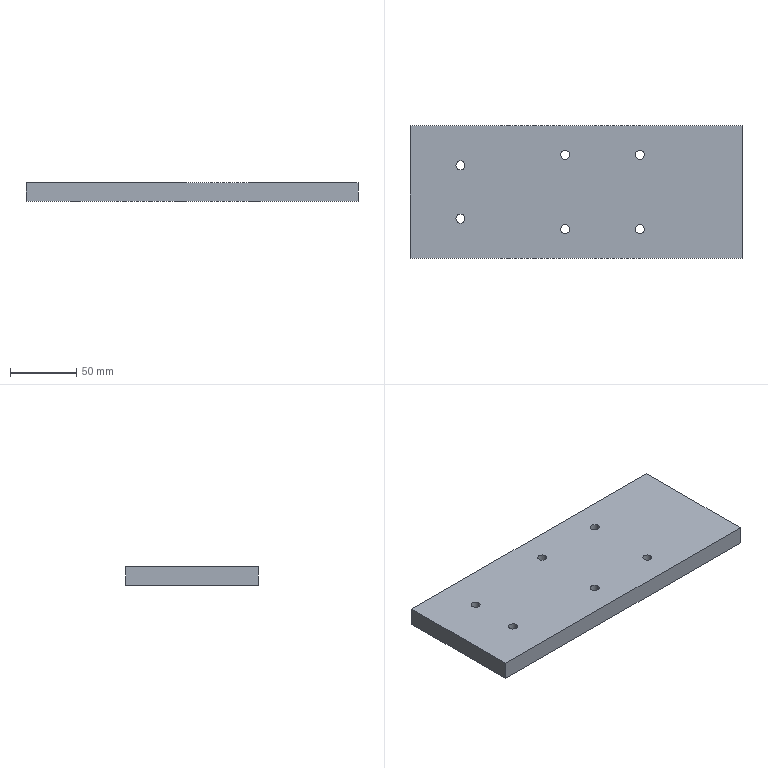Part | SolidWorks | features HoleWzd 2, Extrusion 1 | 1 solid | 18 faces | box 250 x 100 x 14 mm | volume 346949 mm3 | cylinder 12 | plane 6 | commonest cylinder face diameters 6.8 x12
STEP:
#1=CARTESIAN_POINT('',(34.6,70.,0.));
#2=VERTEX_POINT('',#1);
#3=CARTESIAN_POINT('',(41.4,70.,0.));
#4=VERTEX_POINT('',#3);
#5=CARTESIAN_POINT('',(38.,70.,0.));
#6=DIRECTION('',(0.,0.,1.));
#7=DIRECTION('',(1.,0.,0.));
#8=AXIS2_PLACEMENT_3D('',#5,#6,#7);
#9=CIRCLE('',#8,3.4);
#10=EDGE_CURVE('',#2,#4,#9,.T.);
#11=ORIENTED_EDGE('',*,*,#10,.F.);
#12=CARTESIAN_POINT('',(34.6,70.,14.));
#13=VERTEX_POINT('',#12);
#14=CARTESIAN_POINT('',(34.6,70.,14.));
#15=DIRECTION('',(0.,0.,1.));
#16=VECTOR('',#15,1000.);
#17=LINE('',#14,#16);
#18=EDGE_CURVE('',#2,#13,#17,.T.);
#19=ORIENTED_EDGE('',*,*,#18,.T.);
#20=CARTESIAN_POINT('',(41.4,70.,14.));
#21=VERTEX_POINT('',#20);
#22=CARTESIAN_POINT('',(38.,70.,14.));
#23=DIRECTION('',(0.,0.,1.));
#24=DIRECTION('',(1.,0.,0.));
#25=AXIS2_PLACEMENT_3D('',#22,#23,#24);
#26=CIRCLE('',#25,3.4);
#27=EDGE_CURVE('',#13,#21,#26,.T.);
#28=ORIENTED_EDGE('',*,*,#27,.T.);
#29=CARTESIAN_POINT('',(41.4,70.,14.));
#30=DIRECTION('',(0.,0.,1.));
#31=VECTOR('',#30,1000.);
#32=LINE('',#29,#31);
#33=EDGE_CURVE('',#4,#21,#32,.T.);
#34=ORIENTED_EDGE('',*,*,#33,.F.);
#35=EDGE_LOOP('',(#11,#19,#28,#34));
#36=FACE_OUTER_BOUND('',#35,.T.);
#37=CARTESIAN_POINT('',(38.,70.,14.));
#38=DIRECTION('',(0.,0.,1.));
#39=DIRECTION('',(1.,0.,0.));
#40=AXIS2_PLACEMENT_3D('',#37,#38,#39);
#41=CYLINDRICAL_SURFACE('',#40,3.4);
#42=ADVANCED_FACE('',(#36),#41,.F.);
#43=CARTESIAN_POINT('',(34.6,30.,0.));
#44=VERTEX_POINT('',#43);
#45=CARTESIAN_POINT('',(41.4,30.,0.));
#46=VERTEX_POINT('',#45);
#47=CARTESIAN_POINT('',(38.,30.,0.));
#48=DIRECTION('',(0.,0.,1.));
#49=DIRECTION('',(1.,0.,0.));
#50=AXIS2_PLACEMENT_3D('',#47,#48,#49);
#51=CIRCLE('',#50,3.4);
#52=EDGE_CURVE('',#44,#46,#51,.T.);
#53=ORIENTED_EDGE('',*,*,#52,.F.);
#54=CARTESIAN_POINT('',(34.6,30.,14.));
#55=VERTEX_POINT('',#54);
#56=CARTESIAN_POINT('',(34.6,30.,14.));
#57=DIRECTION('',(0.,0.,1.));
#58=VECTOR('',#57,1000.);
#59=LINE('',#56,#58);
#60=EDGE_CURVE('',#44,#55,#59,.T.);
#61=ORIENTED_EDGE('',*,*,#60,.T.);
#62=CARTESIAN_POINT('',(41.4,30.,14.));
#63=VERTEX_POINT('',#62);
#64=CARTESIAN_POINT('',(38.,30.,14.));
#65=DIRECTION('',(0.,0.,1.));
#66=DIRECTION('',(1.,0.,0.));
#67=AXIS2_PLACEMENT_3D('',#64,#65,#66);
#68=CIRCLE('',#67,3.4);
#69=EDGE_CURVE('',#55,#63,#68,.T.);
#70=ORIENTED_EDGE('',*,*,#69,.T.);
#71=CARTESIAN_POINT('',(41.4,30.,14.));
#72=DIRECTION('',(0.,0.,1.));
#73=VECTOR('',#72,1000.);
#74=LINE('',#71,#73);
#75=EDGE_CURVE('',#46,#63,#74,.T.);
#76=ORIENTED_EDGE('',*,*,#75,.F.);
#77=EDGE_LOOP('',(#53,#61,#70,#76));
#78=FACE_OUTER_BOUND('',#77,.T.);
#79=CARTESIAN_POINT('',(38.,30.,14.));
#80=DIRECTION('',(0.,0.,1.));
#81=DIRECTION('',(1.,0.,0.));
#82=AXIS2_PLACEMENT_3D('',#79,#80,#81);
#83=CYLINDRICAL_SURFACE('',#82,3.4);
#84=ADVANCED_FACE('',(#78),#83,.F.);
#85=CARTESIAN_POINT('',(120.4,78.,0.));
#86=VERTEX_POINT('',#85);
#87=CARTESIAN_POINT('',(113.6,78.,0.));
#88=VERTEX_POINT('',#87);
#89=CARTESIAN_POINT('',(117.,78.,0.));
#90=DIRECTION('',(0.,0.,-1.));
#91=DIRECTION('',(-1.,0.,0.));
#92=AXIS2_PLACEMENT_3D('',#89,#90,#91);
#93=CIRCLE('',#92,3.4);
#94=EDGE_CURVE('',#86,#88,#93,.T.);
#95=ORIENTED_EDGE('',*,*,#94,.T.);
#96=CARTESIAN_POINT('',(113.6,78.,14.));
#97=VERTEX_POINT('',#96);
#98=CARTESIAN_POINT('',(113.6,78.,14.));
#99=DIRECTION('',(0.,0.,1.));
#100=VECTOR('',#99,1000.);
#101=LINE('',#98,#100);
#102=EDGE_CURVE('',#88,#97,#101,.T.);
#103=ORIENTED_EDGE('',*,*,#102,.T.);
#104=CARTESIAN_POINT('',(120.4,78.,14.));
#105=VERTEX_POINT('',#104);
#106=CARTESIAN_POINT('',(117.,78.,14.));
#107=DIRECTION('',(0.,0.,1.));
#108=DIRECTION('',(1.,0.,0.));
#109=AXIS2_PLACEMENT_3D('',#106,#107,#108);
#110=CIRCLE('',#109,3.4);
#111=EDGE_CURVE('',#97,#105,#110,.T.);
#112=ORIENTED_EDGE('',*,*,#111,.T.);
#113=CARTESIAN_POINT('',(120.4,78.,14.));
#114=DIRECTION('',(0.,0.,1.));
#115=VECTOR('',#114,1000.);
#116=LINE('',#113,#115);
#117=EDGE_CURVE('',#86,#105,#116,.T.);
#118=ORIENTED_EDGE('',*,*,#117,.F.);
#119=EDGE_LOOP('',(#95,#103,#112,#118));
#120=FACE_OUTER_BOUND('',#119,.T.);
#121=CARTESIAN_POINT('',(117.,78.,14.));
#122=DIRECTION('',(0.,0.,1.));
#123=DIRECTION('',(1.,0.,0.));
#124=AXIS2_PLACEMENT_3D('',#121,#122,#123);
#125=CYLINDRICAL_SURFACE('',#124,3.4);
#126=ADVANCED_FACE('',(#120),#125,.F.);
#127=CARTESIAN_POINT('',(176.4,78.,0.));
#128=VERTEX_POINT('',#127);
#129=CARTESIAN_POINT('',(169.6,78.,0.));
#130=VERTEX_POINT('',#129);
#131=CARTESIAN_POINT('',(173.,78.,0.));
#132=DIRECTION('',(0.,0.,-1.));
#133=DIRECTION('',(-1.,0.,0.));
#134=AXIS2_PLACEMENT_3D('',#131,#132,#133);
#135=CIRCLE('',#134,3.4);
#136=EDGE_CURVE('',#128,#130,#135,.T.);
#137=ORIENTED_EDGE('',*,*,#136,.T.);
#138=CARTESIAN_POINT('',(169.6,78.,14.));
#139=VERTEX_POINT('',#138);
#140=CARTESIAN_POINT('',(169.6,78.,14.));
#141=DIRECTION('',(0.,0.,1.));
#142=VECTOR('',#141,1000.);
#143=LINE('',#140,#142);
#144=EDGE_CURVE('',#130,#139,#143,.T.);
#145=ORIENTED_EDGE('',*,*,#144,.T.);
#146=CARTESIAN_POINT('',(176.4,78.,14.));
#147=VERTEX_POINT('',#146);
#148=CARTESIAN_POINT('',(173.,78.,14.));
#149=DIRECTION('',(0.,0.,1.));
#150=DIRECTION('',(1.,0.,0.));
#151=AXIS2_PLACEMENT_3D('',#148,#149,#150);
#152=CIRCLE('',#151,3.4);
#153=EDGE_CURVE('',#139,#147,#152,.T.);
#154=ORIENTED_EDGE('',*,*,#153,.T.);
#155=CARTESIAN_POINT('',(176.4,78.,14.));
#156=DIRECTION('',(0.,0.,1.));
#157=VECTOR('',#156,1000.);
#158=LINE('',#155,#157);
#159=EDGE_CURVE('',#128,#147,#158,.T.);
#160=ORIENTED_EDGE('',*,*,#159,.F.);
#161=EDGE_LOOP('',(#137,#145,#154,#160));
#162=FACE_OUTER_BOUND('',#161,.T.);
#163=CARTESIAN_POINT('',(173.,78.,14.));
#164=DIRECTION('',(0.,0.,1.));
#165=DIRECTION('',(1.,0.,0.));
#166=AXIS2_PLACEMENT_3D('',#163,#164,#165);
#167=CYLINDRICAL_SURFACE('',#166,3.4);
#168=ADVANCED_FACE('',(#162),#167,.F.);
#169=CARTESIAN_POINT('',(120.4,22.,0.));
#170=VERTEX_POINT('',#169);
#171=CARTESIAN_POINT('',(113.6,22.,0.));
#172=VERTEX_POINT('',#171);
#173=CARTESIAN_POINT('',(117.,22.,0.));
#174=DIRECTION('',(0.,0.,-1.));
#175=DIRECTION('',(-1.,0.,0.));
#176=AXIS2_PLACEMENT_3D('',#173,#174,#175);
#177=CIRCLE('',#176,3.4);
#178=EDGE_CURVE('',#170,#172,#177,.T.);
#179=ORIENTED_EDGE('',*,*,#178,.T.);
#180=CARTESIAN_POINT('',(113.6,22.,14.));
#181=VERTEX_POINT('',#180);
#182=CARTESIAN_POINT('',(113.6,22.,14.));
#183=DIRECTION('',(0.,0.,1.));
#184=VECTOR('',#183,1000.);
#185=LINE('',#182,#184);
#186=EDGE_CURVE('',#172,#181,#185,.T.);
#187=ORIENTED_EDGE('',*,*,#186,.T.);
#188=CARTESIAN_POINT('',(120.4,22.,14.));
#189=VERTEX_POINT('',#188);
#190=CARTESIAN_POINT('',(117.,22.,14.));
#191=DIRECTION('',(0.,0.,1.));
#192=DIRECTION('',(1.,0.,0.));
#193=AXIS2_PLACEMENT_3D('',#190,#191,#192);
#194=CIRCLE('',#193,3.4);
#195=EDGE_CURVE('',#181,#189,#194,.T.);
#196=ORIENTED_EDGE('',*,*,#195,.T.);
#197=CARTESIAN_POINT('',(120.4,22.,14.));
#198=DIRECTION('',(0.,0.,1.));
#199=VECTOR('',#198,1000.);
#200=LINE('',#197,#199);
#201=EDGE_CURVE('',#170,#189,#200,.T.);
#202=ORIENTED_EDGE('',*,*,#201,.F.);
#203=EDGE_LOOP('',(#179,#187,#196,#202));
#204=FACE_OUTER_BOUND('',#203,.T.);
#205=CARTESIAN_POINT('',(117.,22.,14.));
#206=DIRECTION('',(0.,0.,1.));
#207=DIRECTION('',(1.,0.,0.));
#208=AXIS2_PLACEMENT_3D('',#205,#206,#207);
#209=CYLINDRICAL_SURFACE('',#208,3.4);
#210=ADVANCED_FACE('',(#204),#209,.F.);
#211=CARTESIAN_POINT('',(176.4,22.,0.));
#212=VERTEX_POINT('',#211);
#213=CARTESIAN_POINT('',(169.6,22.,0.));
#214=VERTEX_POINT('',#213);
#215=CARTESIAN_POINT('',(173.,22.,0.));
#216=DIRECTION('',(0.,0.,-1.));
#217=DIRECTION('',(-1.,0.,0.));
#218=AXIS2_PLACEMENT_3D('',#215,#216,#217);
#219=CIRCLE('',#218,3.4);
#220=EDGE_CURVE('',#212,#214,#219,.T.);
#221=ORIENTED_EDGE('',*,*,#220,.T.);
#222=CARTESIAN_POINT('',(169.6,22.,14.));
#223=VERTEX_POINT('',#222);
#224=CARTESIAN_POINT('',(169.6,22.,14.));
#225=DIRECTION('',(0.,0.,1.));
#226=VECTOR('',#225,1000.);
#227=LINE('',#224,#226);
#228=EDGE_CURVE('',#214,#223,#227,.T.);
#229=ORIENTED_EDGE('',*,*,#228,.T.);
#230=CARTESIAN_POINT('',(176.4,22.,14.));
#231=VERTEX_POINT('',#230);
#232=CARTESIAN_POINT('',(173.,22.,14.));
#233=DIRECTION('',(0.,0.,1.));
#234=DIRECTION('',(1.,0.,0.));
#235=AXIS2_PLACEMENT_3D('',#232,#233,#234);
#236=CIRCLE('',#235,3.4);
#237=EDGE_CURVE('',#223,#231,#236,.T.);
#238=ORIENTED_EDGE('',*,*,#237,.T.);
#239=CARTESIAN_POINT('',(176.4,22.,14.));
#240=DIRECTION('',(0.,0.,1.));
#241=VECTOR('',#240,1000.);
#242=LINE('',#239,#241);
#243=EDGE_CURVE('',#212,#231,#242,.T.);
#244=ORIENTED_EDGE('',*,*,#243,.F.);
#245=EDGE_LOOP('',(#221,#229,#238,#244));
#246=FACE_OUTER_BOUND('',#245,.T.);
#247=CARTESIAN_POINT('',(173.,22.,14.));
#248=DIRECTION('',(0.,0.,1.));
#249=DIRECTION('',(1.,0.,0.));
#250=AXIS2_PLACEMENT_3D('',#247,#248,#249);
#251=CYLINDRICAL_SURFACE('',#250,3.4);
#252=ADVANCED_FACE('',(#246),#251,.F.);
#253=CARTESIAN_POINT('',(38.,70.,14.));
#254=DIRECTION('',(0.,0.,1.));
#255=DIRECTION('',(1.,0.,0.));
#256=AXIS2_PLACEMENT_3D('',#253,#254,#255);
#257=CIRCLE('',#256,3.4);
#258=EDGE_CURVE('',#21,#13,#257,.T.);
#259=ORIENTED_EDGE('',*,*,#258,.F.);
#260=ORIENTED_EDGE('',*,*,#27,.F.);
#261=EDGE_LOOP('',(#259,#260));
#262=FACE_BOUND('',#261,.T.);
#263=CARTESIAN_POINT('',(38.,30.,14.));
#264=DIRECTION('',(0.,0.,1.));
#265=DIRECTION('',(1.,0.,0.));
#266=AXIS2_PLACEMENT_3D('',#263,#264,#265);
#267=CIRCLE('',#266,3.4);
#268=EDGE_CURVE('',#63,#55,#267,.T.);
#269=ORIENTED_EDGE('',*,*,#268,.F.);
#270=ORIENTED_EDGE('',*,*,#69,.F.);
#271=EDGE_LOOP('',(#269,#270));
#272=FACE_BOUND('',#271,.T.);
#273=CARTESIAN_POINT('',(117.,78.,14.));
#274=DIRECTION('',(0.,0.,1.));
#275=DIRECTION('',(1.,0.,0.));
#276=AXIS2_PLACEMENT_3D('',#273,#274,#275);
#277=CIRCLE('',#276,3.4);
#278=EDGE_CURVE('',#105,#97,#277,.T.);
#279=ORIENTED_EDGE('',*,*,#278,.F.);
#280=ORIENTED_EDGE('',*,*,#111,.F.);
#281=EDGE_LOOP('',(#279,#280));
#282=FACE_BOUND('',#281,.T.);
#283=CARTESIAN_POINT('',(173.,78.,14.));
#284=DIRECTION('',(0.,0.,1.));
#285=DIRECTION('',(1.,0.,0.));
#286=AXIS2_PLACEMENT_3D('',#283,#284,#285);
#287=CIRCLE('',#286,3.4);
#288=EDGE_CURVE('',#147,#139,#287,.T.);
#289=ORIENTED_EDGE('',*,*,#288,.F.);
#290=ORIENTED_EDGE('',*,*,#153,.F.);
#291=EDGE_LOOP('',(#289,#290));
#292=FACE_BOUND('',#291,.T.);
#293=CARTESIAN_POINT('',(117.,22.,14.));
#294=DIRECTION('',(0.,0.,1.));
#295=DIRECTION('',(1.,0.,0.));
#296=AXIS2_PLACEMENT_3D('',#293,#294,#295);
#297=CIRCLE('',#296,3.4);
#298=EDGE_CURVE('',#189,#181,#297,.T.);
#299=ORIENTED_EDGE('',*,*,#298,.F.);
#300=ORIENTED_EDGE('',*,*,#195,.F.);
#301=EDGE_LOOP('',(#299,#300));
#302=FACE_BOUND('',#301,.T.);
#303=CARTESIAN_POINT('',(173.,22.,14.));
#304=DIRECTION('',(0.,0.,1.));
#305=DIRECTION('',(1.,0.,0.));
#306=AXIS2_PLACEMENT_3D('',#303,#304,#305);
#307=CIRCLE('',#306,3.4);
#308=EDGE_CURVE('',#231,#223,#307,.T.);
#309=ORIENTED_EDGE('',*,*,#308,.F.);
#310=ORIENTED_EDGE('',*,*,#237,.F.);
#311=EDGE_LOOP('',(#309,#310));
#312=FACE_BOUND('',#311,.T.);
#313=CARTESIAN_POINT('',(0.,100.,14.));
#314=VERTEX_POINT('',#313);
#315=CARTESIAN_POINT('',(0.,0.,14.));
#316=VERTEX_POINT('',#315);
#317=CARTESIAN_POINT('',(0.,0.,14.));
#318=DIRECTION('',(0.,-1.,0.));
#319=VECTOR('',#318,1000.);
#320=LINE('',#317,#319);
#321=EDGE_CURVE('',#314,#316,#320,.T.);
#322=ORIENTED_EDGE('',*,*,#321,.T.);
#323=CARTESIAN_POINT('',(250.,0.,14.));
#324=VERTEX_POINT('',#323);
#325=CARTESIAN_POINT('',(0.,0.,14.));
#326=DIRECTION('',(1.,0.,0.));
#327=VECTOR('',#326,1000.);
#328=LINE('',#325,#327);
#329=EDGE_CURVE('',#316,#324,#328,.T.);
#330=ORIENTED_EDGE('',*,*,#329,.T.);
#331=CARTESIAN_POINT('',(250.,100.,14.));
#332=VERTEX_POINT('',#331);
#333=CARTESIAN_POINT('',(250.,0.,14.));
#334=DIRECTION('',(0.,1.,0.));
#335=VECTOR('',#334,1000.);
#336=LINE('',#333,#335);
#337=EDGE_CURVE('',#324,#332,#336,.T.);
#338=ORIENTED_EDGE('',*,*,#337,.T.);
#339=CARTESIAN_POINT('',(0.,100.,14.));
#340=DIRECTION('',(-1.,0.,0.));
#341=VECTOR('',#340,1000.);
#342=LINE('',#339,#341);
#343=EDGE_CURVE('',#332,#314,#342,.T.);
#344=ORIENTED_EDGE('',*,*,#343,.T.);
#345=EDGE_LOOP('',(#322,#330,#338,#344));
#346=FACE_OUTER_BOUND('',#345,.T.);
#347=CARTESIAN_POINT('',(0.,0.,14.));
#348=DIRECTION('',(0.,0.,-1.));
#349=DIRECTION('',(-1.,0.,0.));
#350=AXIS2_PLACEMENT_3D('',#347,#348,#349);
#351=PLANE('',#350);
#352=ADVANCED_FACE('',(#262,#272,#282,#292,#302,#312,#346),#351,.F.);
#353=CARTESIAN_POINT('',(38.,70.,0.));
#354=DIRECTION('',(0.,0.,1.));
#355=DIRECTION('',(1.,0.,0.));
#356=AXIS2_PLACEMENT_3D('',#353,#354,#355);
#357=CIRCLE('',#356,3.4);
#358=EDGE_CURVE('',#4,#2,#357,.T.);
#359=ORIENTED_EDGE('',*,*,#358,.T.);
#360=ORIENTED_EDGE('',*,*,#10,.T.);
#361=EDGE_LOOP('',(#359,#360));
#362=FACE_BOUND('',#361,.T.);
#363=CARTESIAN_POINT('',(38.,30.,0.));
#364=DIRECTION('',(0.,0.,1.));
#365=DIRECTION('',(1.,0.,0.));
#366=AXIS2_PLACEMENT_3D('',#363,#364,#365);
#367=CIRCLE('',#366,3.4);
#368=EDGE_CURVE('',#46,#44,#367,.T.);
#369=ORIENTED_EDGE('',*,*,#368,.T.);
#370=ORIENTED_EDGE('',*,*,#52,.T.);
#371=EDGE_LOOP('',(#369,#370));
#372=FACE_BOUND('',#371,.T.);
#373=ORIENTED_EDGE('',*,*,#94,.F.);
#374=CARTESIAN_POINT('',(117.,78.,0.));
#375=DIRECTION('',(0.,0.,-1.));
#376=DIRECTION('',(-1.,0.,0.));
#377=AXIS2_PLACEMENT_3D('',#374,#375,#376);
#378=CIRCLE('',#377,3.4);
#379=EDGE_CURVE('',#88,#86,#378,.T.);
#380=ORIENTED_EDGE('',*,*,#379,.F.);
#381=EDGE_LOOP('',(#373,#380));
#382=FACE_BOUND('',#381,.T.);
#383=ORIENTED_EDGE('',*,*,#136,.F.);
#384=CARTESIAN_POINT('',(173.,78.,0.));
#385=DIRECTION('',(0.,0.,-1.));
#386=DIRECTION('',(-1.,0.,0.));
#387=AXIS2_PLACEMENT_3D('',#384,#385,#386);
#388=CIRCLE('',#387,3.4);
#389=EDGE_CURVE('',#130,#128,#388,.T.);
#390=ORIENTED_EDGE('',*,*,#389,.F.);
#391=EDGE_LOOP('',(#383,#390));
#392=FACE_BOUND('',#391,.T.);
#393=ORIENTED_EDGE('',*,*,#178,.F.);
#394=CARTESIAN_POINT('',(117.,22.,0.));
#395=DIRECTION('',(0.,0.,-1.));
#396=DIRECTION('',(-1.,0.,0.));
#397=AXIS2_PLACEMENT_3D('',#394,#395,#396);
#398=CIRCLE('',#397,3.4);
#399=EDGE_CURVE('',#172,#170,#398,.T.);
#400=ORIENTED_EDGE('',*,*,#399,.F.);
#401=EDGE_LOOP('',(#393,#400));
#402=FACE_BOUND('',#401,.T.);
#403=ORIENTED_EDGE('',*,*,#220,.F.);
#404=CARTESIAN_POINT('',(173.,22.,0.));
#405=DIRECTION('',(0.,0.,-1.));
#406=DIRECTION('',(-1.,0.,0.));
#407=AXIS2_PLACEMENT_3D('',#404,#405,#406);
#408=CIRCLE('',#407,3.4);
#409=EDGE_CURVE('',#214,#212,#408,.T.);
#410=ORIENTED_EDGE('',*,*,#409,.F.);
#411=EDGE_LOOP('',(#403,#410));
#412=FACE_BOUND('',#411,.T.);
#413=CARTESIAN_POINT('',(0.,100.,0.));
#414=VERTEX_POINT('',#413);
#415=CARTESIAN_POINT('',(0.,0.,0.));
#416=VERTEX_POINT('',#415);
#417=CARTESIAN_POINT('',(0.,0.,0.));
#418=DIRECTION('',(0.,-1.,0.));
#419=VECTOR('',#418,1000.);
#420=LINE('',#417,#419);
#421=EDGE_CURVE('',#414,#416,#420,.T.);
#422=ORIENTED_EDGE('',*,*,#421,.F.);
#423=CARTESIAN_POINT('',(250.,100.,0.));
#424=VERTEX_POINT('',#423);
#425=CARTESIAN_POINT('',(0.,100.,0.));
#426=DIRECTION('',(-1.,0.,0.));
#427=VECTOR('',#426,1000.);
#428=LINE('',#425,#427);
#429=EDGE_CURVE('',#424,#414,#428,.T.);
#430=ORIENTED_EDGE('',*,*,#429,.F.);
#431=CARTESIAN_POINT('',(250.,0.,0.));
#432=VERTEX_POINT('',#431);
#433=CARTESIAN_POINT('',(250.,0.,0.));
#434=DIRECTION('',(0.,1.,0.));
#435=VECTOR('',#434,1000.);
#436=LINE('',#433,#435);
#437=EDGE_CURVE('',#432,#424,#436,.T.);
#438=ORIENTED_EDGE('',*,*,#437,.F.);
#439=CARTESIAN_POINT('',(0.,0.,0.));
#440=DIRECTION('',(1.,0.,0.));
#441=VECTOR('',#440,1000.);
#442=LINE('',#439,#441);
#443=EDGE_CURVE('',#416,#432,#442,.T.);
#444=ORIENTED_EDGE('',*,*,#443,.F.);
#445=EDGE_LOOP('',(#422,#430,#438,#444));
#446=FACE_OUTER_BOUND('',#445,.T.);
#447=CARTESIAN_POINT('',(0.,0.,0.));
#448=DIRECTION('',(0.,0.,-1.));
#449=DIRECTION('',(-1.,0.,0.));
#450=AXIS2_PLACEMENT_3D('',#447,#448,#449);
#451=PLANE('',#450);
#452=ADVANCED_FACE('',(#362,#372,#382,#392,#402,#412,#446),#451,.T.);
#453=ORIENTED_EDGE('',*,*,#421,.T.);
#454=CARTESIAN_POINT('',(0.,0.,14.));
#455=DIRECTION('',(0.,0.,-1.));
#456=VECTOR('',#455,1000.);
#457=LINE('',#454,#456);
#458=EDGE_CURVE('',#316,#416,#457,.T.);
#459=ORIENTED_EDGE('',*,*,#458,.F.);
#460=ORIENTED_EDGE('',*,*,#321,.F.);
#461=CARTESIAN_POINT('',(0.,100.,14.));
#462=DIRECTION('',(0.,0.,-1.));
#463=VECTOR('',#462,1000.);
#464=LINE('',#461,#463);
#465=EDGE_CURVE('',#314,#414,#464,.T.);
#466=ORIENTED_EDGE('',*,*,#465,.T.);
#467=EDGE_LOOP('',(#453,#459,#460,#466));
#468=FACE_OUTER_BOUND('',#467,.T.);
#469=CARTESIAN_POINT('',(0.,0.,14.));
#470=DIRECTION('',(1.,0.,0.));
#471=DIRECTION('',(0.,0.,-1.));
#472=AXIS2_PLACEMENT_3D('',#469,#470,#471);
#473=PLANE('',#472);
#474=ADVANCED_FACE('',(#468),#473,.F.);
#475=ORIENTED_EDGE('',*,*,#443,.T.);
#476=CARTESIAN_POINT('',(250.,0.,14.));
#477=DIRECTION('',(0.,0.,-1.));
#478=VECTOR('',#477,1000.);
#479=LINE('',#476,#478);
#480=EDGE_CURVE('',#324,#432,#479,.T.);
#481=ORIENTED_EDGE('',*,*,#480,.F.);
#482=ORIENTED_EDGE('',*,*,#329,.F.);
#483=ORIENTED_EDGE('',*,*,#458,.T.);
#484=EDGE_LOOP('',(#475,#481,#482,#483));
#485=FACE_OUTER_BOUND('',#484,.T.);
#486=CARTESIAN_POINT('',(0.,0.,14.));
#487=DIRECTION('',(0.,1.,0.));
#488=DIRECTION('',(0.,0.,1.));
#489=AXIS2_PLACEMENT_3D('',#486,#487,#488);
#490=PLANE('',#489);
#491=ADVANCED_FACE('',(#485),#490,.F.);
#492=ORIENTED_EDGE('',*,*,#437,.T.);
#493=CARTESIAN_POINT('',(250.,100.,14.));
#494=DIRECTION('',(0.,0.,-1.));
#495=VECTOR('',#494,1000.);
#496=LINE('',#493,#495);
#497=EDGE_CURVE('',#332,#424,#496,.T.);
#498=ORIENTED_EDGE('',*,*,#497,.F.);
#499=ORIENTED_EDGE('',*,*,#337,.F.);
#500=ORIENTED_EDGE('',*,*,#480,.T.);
#501=EDGE_LOOP('',(#492,#498,#499,#500));
#502=FACE_OUTER_BOUND('',#501,.T.);
#503=CARTESIAN_POINT('',(250.,0.,14.));
#504=DIRECTION('',(-1.,0.,0.));
#505=DIRECTION('',(0.,0.,1.));
#506=AXIS2_PLACEMENT_3D('',#503,#504,#505);
#507=PLANE('',#506);
#508=ADVANCED_FACE('',(#502),#507,.F.);
#509=ORIENTED_EDGE('',*,*,#429,.T.);
#510=ORIENTED_EDGE('',*,*,#465,.F.);
#511=ORIENTED_EDGE('',*,*,#343,.F.);
#512=ORIENTED_EDGE('',*,*,#497,.T.);
#513=EDGE_LOOP('',(#509,#510,#511,#512));
#514=FACE_OUTER_BOUND('',#513,.T.);
#515=CARTESIAN_POINT('',(0.,100.,14.));
#516=DIRECTION('',(0.,-1.,0.));
#517=DIRECTION('',(0.,0.,-1.));
#518=AXIS2_PLACEMENT_3D('',#515,#516,#517);
#519=PLANE('',#518);
#520=ADVANCED_FACE('',(#514),#519,.F.);
#521=ORIENTED_EDGE('',*,*,#228,.F.);
#522=ORIENTED_EDGE('',*,*,#409,.T.);
#523=ORIENTED_EDGE('',*,*,#243,.T.);
#524=ORIENTED_EDGE('',*,*,#308,.T.);
#525=EDGE_LOOP('',(#521,#522,#523,#524));
#526=FACE_OUTER_BOUND('',#525,.T.);
#527=CARTESIAN_POINT('',(173.,22.,14.));
#528=DIRECTION('',(0.,0.,1.));
#529=DIRECTION('',(1.,0.,0.));
#530=AXIS2_PLACEMENT_3D('',#527,#528,#529);
#531=CYLINDRICAL_SURFACE('',#530,3.4);
#532=ADVANCED_FACE('',(#526),#531,.F.);
#533=ORIENTED_EDGE('',*,*,#186,.F.);
#534=ORIENTED_EDGE('',*,*,#399,.T.);
#535=ORIENTED_EDGE('',*,*,#201,.T.);
#536=ORIENTED_EDGE('',*,*,#298,.T.);
#537=EDGE_LOOP('',(#533,#534,#535,#536));
#538=FACE_OUTER_BOUND('',#537,.T.);
#539=CARTESIAN_POINT('',(117.,22.,14.));
#540=DIRECTION('',(0.,0.,1.));
#541=DIRECTION('',(1.,0.,0.));
#542=AXIS2_PLACEMENT_3D('',#539,#540,#541);
#543=CYLINDRICAL_SURFACE('',#542,3.4);
#544=ADVANCED_FACE('',(#538),#543,.F.);
#545=ORIENTED_EDGE('',*,*,#144,.F.);
#546=ORIENTED_EDGE('',*,*,#389,.T.);
#547=ORIENTED_EDGE('',*,*,#159,.T.);
#548=ORIENTED_EDGE('',*,*,#288,.T.);
#549=EDGE_LOOP('',(#545,#546,#547,#548));
#550=FACE_OUTER_BOUND('',#549,.T.);
#551=CARTESIAN_POINT('',(173.,78.,14.));
#552=DIRECTION('',(0.,0.,1.));
#553=DIRECTION('',(1.,0.,0.));
#554=AXIS2_PLACEMENT_3D('',#551,#552,#553);
#555=CYLINDRICAL_SURFACE('',#554,3.4);
#556=ADVANCED_FACE('',(#550),#555,.F.);
#557=ORIENTED_EDGE('',*,*,#102,.F.);
#558=ORIENTED_EDGE('',*,*,#379,.T.);
#559=ORIENTED_EDGE('',*,*,#117,.T.);
#560=ORIENTED_EDGE('',*,*,#278,.T.);
#561=EDGE_LOOP('',(#557,#558,#559,#560));
#562=FACE_OUTER_BOUND('',#561,.T.);
#563=CARTESIAN_POINT('',(117.,78.,14.));
#564=DIRECTION('',(0.,0.,1.));
#565=DIRECTION('',(1.,0.,0.));
#566=AXIS2_PLACEMENT_3D('',#563,#564,#565);
#567=CYLINDRICAL_SURFACE('',#566,3.4);
#568=ADVANCED_FACE('',(#562),#567,.F.);
#569=ORIENTED_EDGE('',*,*,#60,.F.);
#570=ORIENTED_EDGE('',*,*,#368,.F.);
#571=ORIENTED_EDGE('',*,*,#75,.T.);
#572=ORIENTED_EDGE('',*,*,#268,.T.);
#573=EDGE_LOOP('',(#569,#570,#571,#572));
#574=FACE_OUTER_BOUND('',#573,.T.);
#575=CARTESIAN_POINT('',(38.,30.,14.));
#576=DIRECTION('',(0.,0.,1.));
#577=DIRECTION('',(1.,0.,0.));
#578=AXIS2_PLACEMENT_3D('',#575,#576,#577);
#579=CYLINDRICAL_SURFACE('',#578,3.4);
#580=ADVANCED_FACE('',(#574),#579,.F.);
#581=ORIENTED_EDGE('',*,*,#18,.F.);
#582=ORIENTED_EDGE('',*,*,#358,.F.);
#583=ORIENTED_EDGE('',*,*,#33,.T.);
#584=ORIENTED_EDGE('',*,*,#258,.T.);
#585=EDGE_LOOP('',(#581,#582,#583,#584));
#586=FACE_OUTER_BOUND('',#585,.T.);
#587=CARTESIAN_POINT('',(38.,70.,14.));
#588=DIRECTION('',(0.,0.,1.));
#589=DIRECTION('',(1.,0.,0.));
#590=AXIS2_PLACEMENT_3D('',#587,#588,#589);
#591=CYLINDRICAL_SURFACE('',#590,3.4);
#592=ADVANCED_FACE('',(#586),#591,.F.);
#593=CLOSED_SHELL('',(#42,#84,#126,#168,#210,#252,#352,#452,#474,#491,#508,#520,#532,#544,#556,#568,#580,#592));
#594=MANIFOLD_SOLID_BREP('',#593);
#595=CARTESIAN_POINT('',(0.,0.,0.));
#596=DIRECTION('',(0.,0.,1.));
#597=DIRECTION('',(1.,0.,0.));
#598=AXIS2_PLACEMENT_3D('',#595,#596,#597);
#599=(LENGTH_UNIT()NAMED_UNIT(*)SI_UNIT(.MILLI.,.METRE.));
#600=UNCERTAINTY_MEASURE_WITH_UNIT(LENGTH_MEASURE(0.00001),#599,'','');
#601=(NAMED_UNIT(*)PLANE_ANGLE_UNIT()SI_UNIT($,.RADIAN.));
#602=(NAMED_UNIT(*)SI_UNIT($,.STERADIAN.)SOLID_ANGLE_UNIT());
#603=(GEOMETRIC_REPRESENTATION_CONTEXT(3)GLOBAL_UNCERTAINTY_ASSIGNED_CONTEXT((#600))GLOBAL_UNIT_ASSIGNED_CONTEXT((#599,#601,#602))REPRESENTATION_CONTEXT('',''));
#604=ADVANCED_BREP_SHAPE_REPRESENTATION('',(#594,#598),#603);